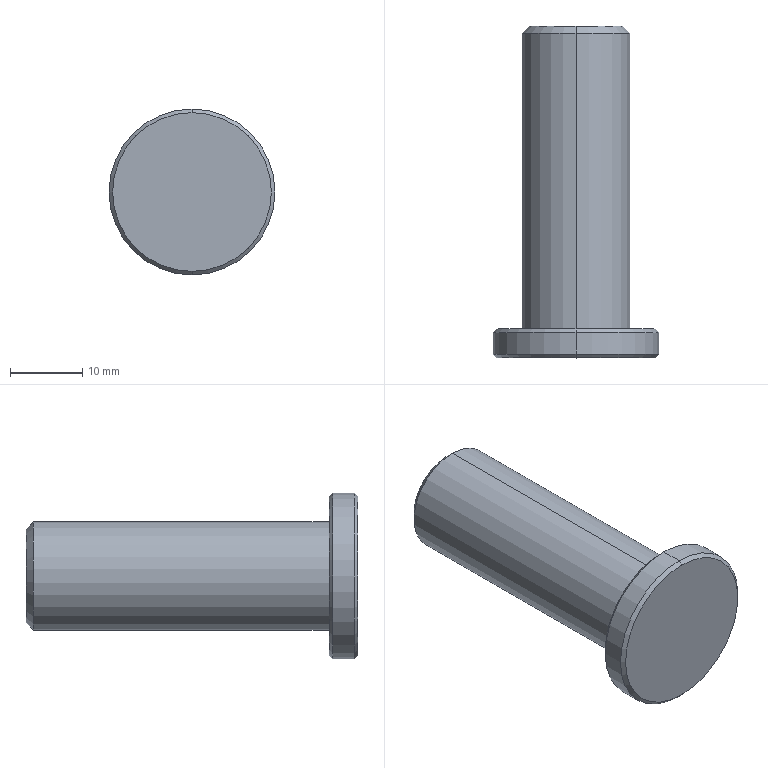Part | SolidWorks | features Chamfer 2, Extrusion 1, ICE 1 | 1 solid | 13 faces | box 23 x 46 x 23 mm | volume 9044 mm3 | cone 6 | cylinder 4 | plane 3 | commonest cylinder face diameters 15 x2 23 x2
STEP:
#1=CARTESIAN_POINT('',(0.,4.,11.));
#2=VERTEX_POINT('',#1);
#3=CARTESIAN_POINT('',(0.,4.,-11.));
#4=VERTEX_POINT('',#3);
#5=CARTESIAN_POINT('',(0.,4.,0.));
#6=DIRECTION('',(0.,1.,0.));
#7=DIRECTION('',(0.,0.,1.));
#8=AXIS2_PLACEMENT_3D('',#5,#6,#7);
#9=CIRCLE('',#8,11.);
#10=EDGE_CURVE('',#2,#4,#9,.T.);
#11=ORIENTED_EDGE('',*,*,#10,.F.);
#12=CARTESIAN_POINT('',(0.,3.5,11.5));
#13=VERTEX_POINT('',#12);
#14=CARTESIAN_POINT('',(0.,4.,11.));
#15=DIRECTION('',(0.,-0.7071,0.7071));
#16=VECTOR('',#15,1000.);
#17=LINE('',#14,#16);
#18=EDGE_CURVE('',#2,#13,#17,.T.);
#19=ORIENTED_EDGE('',*,*,#18,.T.);
#20=CARTESIAN_POINT('',(0.,3.5,-11.5));
#21=VERTEX_POINT('',#20);
#22=CARTESIAN_POINT('',(0.,3.5,0.));
#23=DIRECTION('',(0.,-1.,0.));
#24=DIRECTION('',(0.,0.,1.));
#25=AXIS2_PLACEMENT_3D('',#22,#23,#24);
#26=CIRCLE('',#25,11.5);
#27=EDGE_CURVE('',#21,#13,#26,.T.);
#28=ORIENTED_EDGE('',*,*,#27,.F.);
#29=CARTESIAN_POINT('',(0.,4.,-11.));
#30=DIRECTION('',(0.,-0.7071,-0.7071));
#31=VECTOR('',#30,1000.);
#32=LINE('',#29,#31);
#33=EDGE_CURVE('',#4,#21,#32,.T.);
#34=ORIENTED_EDGE('',*,*,#33,.F.);
#35=EDGE_LOOP('',(#11,#19,#28,#34));
#36=FACE_OUTER_BOUND('',#35,.T.);
#37=CARTESIAN_POINT('',(0.,4.,0.));
#38=DIRECTION('',(0.,-1.,0.));
#39=DIRECTION('',(0.,0.,-1.));
#40=AXIS2_PLACEMENT_3D('',#37,#38,#39);
#41=CONICAL_SURFACE('',#40,11.,0.7854);
#42=ADVANCED_FACE('',(#36),#41,.T.);
#43=CARTESIAN_POINT('',(0.,0.,-11.));
#44=VERTEX_POINT('',#43);
#45=CARTESIAN_POINT('',(0.,0.,11.));
#46=VERTEX_POINT('',#45);
#47=CARTESIAN_POINT('',(0.,0.,0.));
#48=DIRECTION('',(0.,-1.,0.));
#49=DIRECTION('',(0.,0.,1.));
#50=AXIS2_PLACEMENT_3D('',#47,#48,#49);
#51=CIRCLE('',#50,11.);
#52=EDGE_CURVE('',#44,#46,#51,.T.);
#53=ORIENTED_EDGE('',*,*,#52,.F.);
#54=CARTESIAN_POINT('',(0.,0.5,-11.5));
#55=VERTEX_POINT('',#54);
#56=CARTESIAN_POINT('',(0.,0.5,-11.5));
#57=DIRECTION('',(0.,0.7071,-0.7071));
#58=VECTOR('',#57,1000.);
#59=LINE('',#56,#58);
#60=EDGE_CURVE('',#44,#55,#59,.T.);
#61=ORIENTED_EDGE('',*,*,#60,.T.);
#62=CARTESIAN_POINT('',(0.,0.5,11.5));
#63=VERTEX_POINT('',#62);
#64=CARTESIAN_POINT('',(0.,0.5,0.));
#65=DIRECTION('',(0.,1.,0.));
#66=DIRECTION('',(0.,0.,1.));
#67=AXIS2_PLACEMENT_3D('',#64,#65,#66);
#68=CIRCLE('',#67,11.5);
#69=EDGE_CURVE('',#63,#55,#68,.T.);
#70=ORIENTED_EDGE('',*,*,#69,.F.);
#71=CARTESIAN_POINT('',(0.,0.5,11.5));
#72=DIRECTION('',(0.,0.7071,0.7071));
#73=VECTOR('',#72,1000.);
#74=LINE('',#71,#73);
#75=EDGE_CURVE('',#46,#63,#74,.T.);
#76=ORIENTED_EDGE('',*,*,#75,.F.);
#77=EDGE_LOOP('',(#53,#61,#70,#76));
#78=FACE_OUTER_BOUND('',#77,.T.);
#79=CARTESIAN_POINT('',(0.,0.5,0.));
#80=DIRECTION('',(0.,1.,0.));
#81=DIRECTION('',(0.,0.,1.));
#82=AXIS2_PLACEMENT_3D('',#79,#80,#81);
#83=CONICAL_SURFACE('',#82,11.5,0.7854);
#84=ADVANCED_FACE('',(#78),#83,.T.);
#85=CARTESIAN_POINT('',(0.,46.,6.5));
#86=VERTEX_POINT('',#85);
#87=CARTESIAN_POINT('',(0.,46.,-6.5));
#88=VERTEX_POINT('',#87);
#89=CARTESIAN_POINT('',(0.,46.,0.));
#90=DIRECTION('',(0.,1.,0.));
#91=DIRECTION('',(0.,0.,1.));
#92=AXIS2_PLACEMENT_3D('',#89,#90,#91);
#93=CIRCLE('',#92,6.5);
#94=EDGE_CURVE('',#86,#88,#93,.T.);
#95=ORIENTED_EDGE('',*,*,#94,.F.);
#96=CARTESIAN_POINT('',(0.,45.,7.5));
#97=VERTEX_POINT('',#96);
#98=CARTESIAN_POINT('',(0.,46.,6.5));
#99=DIRECTION('',(0.,-0.7071,0.7071));
#100=VECTOR('',#99,1000.);
#101=LINE('',#98,#100);
#102=EDGE_CURVE('',#86,#97,#101,.T.);
#103=ORIENTED_EDGE('',*,*,#102,.T.);
#104=CARTESIAN_POINT('',(0.,45.,-7.5));
#105=VERTEX_POINT('',#104);
#106=CARTESIAN_POINT('',(0.,45.,0.));
#107=DIRECTION('',(0.,-1.,0.));
#108=DIRECTION('',(0.,0.,1.));
#109=AXIS2_PLACEMENT_3D('',#106,#107,#108);
#110=CIRCLE('',#109,7.5);
#111=EDGE_CURVE('',#105,#97,#110,.T.);
#112=ORIENTED_EDGE('',*,*,#111,.F.);
#113=CARTESIAN_POINT('',(0.,46.,-6.5));
#114=DIRECTION('',(0.,-0.7071,-0.7071));
#115=VECTOR('',#114,1000.);
#116=LINE('',#113,#115);
#117=EDGE_CURVE('',#88,#105,#116,.T.);
#118=ORIENTED_EDGE('',*,*,#117,.F.);
#119=EDGE_LOOP('',(#95,#103,#112,#118));
#120=FACE_OUTER_BOUND('',#119,.T.);
#121=CARTESIAN_POINT('',(0.,46.,0.));
#122=DIRECTION('',(0.,-1.,0.));
#123=DIRECTION('',(0.,0.,-1.));
#124=AXIS2_PLACEMENT_3D('',#121,#122,#123);
#125=CONICAL_SURFACE('',#124,6.5,0.7854);
#126=ADVANCED_FACE('',(#120),#125,.T.);
#127=ORIENTED_EDGE('',*,*,#111,.T.);
#128=CARTESIAN_POINT('',(0.,4.,7.5));
#129=VERTEX_POINT('',#128);
#130=CARTESIAN_POINT('',(0.,46.,7.5));
#131=DIRECTION('',(0.,-1.,0.));
#132=VECTOR('',#131,1000.);
#133=LINE('',#130,#132);
#134=EDGE_CURVE('',#97,#129,#133,.T.);
#135=ORIENTED_EDGE('',*,*,#134,.T.);
#136=CARTESIAN_POINT('',(0.,4.,-7.5));
#137=VERTEX_POINT('',#136);
#138=CARTESIAN_POINT('',(0.,4.,0.));
#139=DIRECTION('',(0.,1.,0.));
#140=DIRECTION('',(0.,0.,1.));
#141=AXIS2_PLACEMENT_3D('',#138,#139,#140);
#142=CIRCLE('',#141,7.5);
#143=EDGE_CURVE('',#129,#137,#142,.T.);
#144=ORIENTED_EDGE('',*,*,#143,.T.);
#145=CARTESIAN_POINT('',(0.,46.,-7.5));
#146=DIRECTION('',(0.,-1.,0.));
#147=VECTOR('',#146,1000.);
#148=LINE('',#145,#147);
#149=EDGE_CURVE('',#105,#137,#148,.T.);
#150=ORIENTED_EDGE('',*,*,#149,.F.);
#151=EDGE_LOOP('',(#127,#135,#144,#150));
#152=FACE_OUTER_BOUND('',#151,.T.);
#153=CARTESIAN_POINT('',(0.,46.,0.));
#154=DIRECTION('',(0.,-1.,0.));
#155=DIRECTION('',(0.,0.,-1.));
#156=AXIS2_PLACEMENT_3D('',#153,#154,#155);
#157=CYLINDRICAL_SURFACE('',#156,7.5);
#158=ADVANCED_FACE('',(#152),#157,.T.);
#159=ORIENTED_EDGE('',*,*,#27,.T.);
#160=CARTESIAN_POINT('',(0.,4.,11.5));
#161=DIRECTION('',(0.,-1.,0.));
#162=VECTOR('',#161,1000.);
#163=LINE('',#160,#162);
#164=EDGE_CURVE('',#13,#63,#163,.T.);
#165=ORIENTED_EDGE('',*,*,#164,.T.);
#166=ORIENTED_EDGE('',*,*,#69,.T.);
#167=CARTESIAN_POINT('',(0.,4.,-11.5));
#168=DIRECTION('',(0.,-1.,0.));
#169=VECTOR('',#168,1000.);
#170=LINE('',#167,#169);
#171=EDGE_CURVE('',#21,#55,#170,.T.);
#172=ORIENTED_EDGE('',*,*,#171,.F.);
#173=EDGE_LOOP('',(#159,#165,#166,#172));
#174=FACE_OUTER_BOUND('',#173,.T.);
#175=CARTESIAN_POINT('',(0.,4.,0.));
#176=DIRECTION('',(0.,-1.,0.));
#177=DIRECTION('',(0.,0.,-1.));
#178=AXIS2_PLACEMENT_3D('',#175,#176,#177);
#179=CYLINDRICAL_SURFACE('',#178,11.5);
#180=ADVANCED_FACE('',(#174),#179,.T.);
#181=ORIENTED_EDGE('',*,*,#164,.F.);
#182=CARTESIAN_POINT('',(0.,3.5,0.));
#183=DIRECTION('',(0.,-1.,0.));
#184=DIRECTION('',(0.,0.,1.));
#185=AXIS2_PLACEMENT_3D('',#182,#183,#184);
#186=CIRCLE('',#185,11.5);
#187=EDGE_CURVE('',#13,#21,#186,.T.);
#188=ORIENTED_EDGE('',*,*,#187,.T.);
#189=ORIENTED_EDGE('',*,*,#171,.T.);
#190=CARTESIAN_POINT('',(0.,0.5,0.));
#191=DIRECTION('',(0.,1.,0.));
#192=DIRECTION('',(0.,0.,1.));
#193=AXIS2_PLACEMENT_3D('',#190,#191,#192);
#194=CIRCLE('',#193,11.5);
#195=EDGE_CURVE('',#55,#63,#194,.T.);
#196=ORIENTED_EDGE('',*,*,#195,.T.);
#197=EDGE_LOOP('',(#181,#188,#189,#196));
#198=FACE_OUTER_BOUND('',#197,.T.);
#199=CARTESIAN_POINT('',(0.,4.,0.));
#200=DIRECTION('',(0.,-1.,0.));
#201=DIRECTION('',(0.,0.,-1.));
#202=AXIS2_PLACEMENT_3D('',#199,#200,#201);
#203=CYLINDRICAL_SURFACE('',#202,11.5);
#204=ADVANCED_FACE('',(#198),#203,.T.);
#205=CARTESIAN_POINT('',(0.,4.,0.));
#206=DIRECTION('',(0.,1.,0.));
#207=DIRECTION('',(0.,0.,1.));
#208=AXIS2_PLACEMENT_3D('',#205,#206,#207);
#209=CIRCLE('',#208,11.);
#210=EDGE_CURVE('',#4,#2,#209,.T.);
#211=ORIENTED_EDGE('',*,*,#210,.T.);
#212=ORIENTED_EDGE('',*,*,#10,.T.);
#213=EDGE_LOOP('',(#211,#212));
#214=FACE_OUTER_BOUND('',#213,.T.);
#215=CARTESIAN_POINT('',(0.,4.,0.));
#216=DIRECTION('',(0.,1.,0.));
#217=DIRECTION('',(0.,0.,1.));
#218=AXIS2_PLACEMENT_3D('',#215,#216,#217);
#219=CIRCLE('',#218,7.5);
#220=EDGE_CURVE('',#137,#129,#219,.T.);
#221=ORIENTED_EDGE('',*,*,#220,.F.);
#222=ORIENTED_EDGE('',*,*,#143,.F.);
#223=EDGE_LOOP('',(#221,#222));
#224=FACE_BOUND('',#223,.T.);
#225=CARTESIAN_POINT('',(0.,4.,0.));
#226=DIRECTION('',(0.,1.,0.));
#227=DIRECTION('',(0.,0.,1.));
#228=AXIS2_PLACEMENT_3D('',#225,#226,#227);
#229=PLANE('',#228);
#230=ADVANCED_FACE('',(#214,#224),#229,.T.);
#231=CARTESIAN_POINT('',(0.,0.,0.));
#232=DIRECTION('',(0.,-1.,0.));
#233=DIRECTION('',(0.,0.,1.));
#234=AXIS2_PLACEMENT_3D('',#231,#232,#233);
#235=CIRCLE('',#234,11.);
#236=EDGE_CURVE('',#46,#44,#235,.T.);
#237=ORIENTED_EDGE('',*,*,#236,.T.);
#238=ORIENTED_EDGE('',*,*,#52,.T.);
#239=EDGE_LOOP('',(#237,#238));
#240=FACE_OUTER_BOUND('',#239,.T.);
#241=CARTESIAN_POINT('',(0.,0.,0.));
#242=DIRECTION('',(0.,1.,0.));
#243=DIRECTION('',(0.,0.,1.));
#244=AXIS2_PLACEMENT_3D('',#241,#242,#243);
#245=PLANE('',#244);
#246=ADVANCED_FACE('',(#240),#245,.F.);
#247=ORIENTED_EDGE('',*,*,#134,.F.);
#248=CARTESIAN_POINT('',(0.,45.,0.));
#249=DIRECTION('',(0.,-1.,0.));
#250=DIRECTION('',(0.,0.,1.));
#251=AXIS2_PLACEMENT_3D('',#248,#249,#250);
#252=CIRCLE('',#251,7.5);
#253=EDGE_CURVE('',#97,#105,#252,.T.);
#254=ORIENTED_EDGE('',*,*,#253,.T.);
#255=ORIENTED_EDGE('',*,*,#149,.T.);
#256=ORIENTED_EDGE('',*,*,#220,.T.);
#257=EDGE_LOOP('',(#247,#254,#255,#256));
#258=FACE_OUTER_BOUND('',#257,.T.);
#259=CARTESIAN_POINT('',(0.,46.,0.));
#260=DIRECTION('',(0.,-1.,0.));
#261=DIRECTION('',(0.,0.,-1.));
#262=AXIS2_PLACEMENT_3D('',#259,#260,#261);
#263=CYLINDRICAL_SURFACE('',#262,7.5);
#264=ADVANCED_FACE('',(#258),#263,.T.);
#265=CARTESIAN_POINT('',(0.,46.,0.));
#266=DIRECTION('',(0.,1.,0.));
#267=DIRECTION('',(0.,0.,1.));
#268=AXIS2_PLACEMENT_3D('',#265,#266,#267);
#269=CIRCLE('',#268,6.5);
#270=EDGE_CURVE('',#88,#86,#269,.T.);
#271=ORIENTED_EDGE('',*,*,#270,.T.);
#272=ORIENTED_EDGE('',*,*,#94,.T.);
#273=EDGE_LOOP('',(#271,#272));
#274=FACE_OUTER_BOUND('',#273,.T.);
#275=CARTESIAN_POINT('',(0.,46.,0.));
#276=DIRECTION('',(0.,1.,0.));
#277=DIRECTION('',(0.,0.,1.));
#278=AXIS2_PLACEMENT_3D('',#275,#276,#277);
#279=PLANE('',#278);
#280=ADVANCED_FACE('',(#274),#279,.T.);
#281=ORIENTED_EDGE('',*,*,#102,.F.);
#282=ORIENTED_EDGE('',*,*,#270,.F.);
#283=ORIENTED_EDGE('',*,*,#117,.T.);
#284=ORIENTED_EDGE('',*,*,#253,.F.);
#285=EDGE_LOOP('',(#281,#282,#283,#284));
#286=FACE_OUTER_BOUND('',#285,.T.);
#287=CARTESIAN_POINT('',(0.,46.,0.));
#288=DIRECTION('',(0.,-1.,0.));
#289=DIRECTION('',(0.,0.,-1.));
#290=AXIS2_PLACEMENT_3D('',#287,#288,#289);
#291=CONICAL_SURFACE('',#290,6.5,0.7854);
#292=ADVANCED_FACE('',(#286),#291,.T.);
#293=ORIENTED_EDGE('',*,*,#60,.F.);
#294=ORIENTED_EDGE('',*,*,#236,.F.);
#295=ORIENTED_EDGE('',*,*,#75,.T.);
#296=ORIENTED_EDGE('',*,*,#195,.F.);
#297=EDGE_LOOP('',(#293,#294,#295,#296));
#298=FACE_OUTER_BOUND('',#297,.T.);
#299=CARTESIAN_POINT('',(0.,0.5,0.));
#300=DIRECTION('',(0.,1.,0.));
#301=DIRECTION('',(0.,0.,1.));
#302=AXIS2_PLACEMENT_3D('',#299,#300,#301);
#303=CONICAL_SURFACE('',#302,11.5,0.7854);
#304=ADVANCED_FACE('',(#298),#303,.T.);
#305=ORIENTED_EDGE('',*,*,#18,.F.);
#306=ORIENTED_EDGE('',*,*,#210,.F.);
#307=ORIENTED_EDGE('',*,*,#33,.T.);
#308=ORIENTED_EDGE('',*,*,#187,.F.);
#309=EDGE_LOOP('',(#305,#306,#307,#308));
#310=FACE_OUTER_BOUND('',#309,.T.);
#311=CARTESIAN_POINT('',(0.,4.,0.));
#312=DIRECTION('',(0.,-1.,0.));
#313=DIRECTION('',(0.,0.,-1.));
#314=AXIS2_PLACEMENT_3D('',#311,#312,#313);
#315=CONICAL_SURFACE('',#314,11.,0.7854);
#316=ADVANCED_FACE('',(#310),#315,.T.);
#317=CLOSED_SHELL('',(#42,#84,#126,#158,#180,#204,#230,#246,#264,#280,#292,#304,#316));
#318=MANIFOLD_SOLID_BREP('',#317);
#319=CARTESIAN_POINT('',(0.,0.,0.));
#320=DIRECTION('',(0.,0.,1.));
#321=DIRECTION('',(1.,0.,0.));
#322=AXIS2_PLACEMENT_3D('',#319,#320,#321);
#323=(LENGTH_UNIT()NAMED_UNIT(*)SI_UNIT(.MILLI.,.METRE.));
#324=UNCERTAINTY_MEASURE_WITH_UNIT(LENGTH_MEASURE(0.00001),#323,'','');
#325=(NAMED_UNIT(*)PLANE_ANGLE_UNIT()SI_UNIT($,.RADIAN.));
#326=(NAMED_UNIT(*)SI_UNIT($,.STERADIAN.)SOLID_ANGLE_UNIT());
#327=(GEOMETRIC_REPRESENTATION_CONTEXT(3)GLOBAL_UNCERTAINTY_ASSIGNED_CONTEXT((#324))GLOBAL_UNIT_ASSIGNED_CONTEXT((#323,#325,#326))REPRESENTATION_CONTEXT('',''));
#328=ADVANCED_BREP_SHAPE_REPRESENTATION('',(#318,#322),#327);